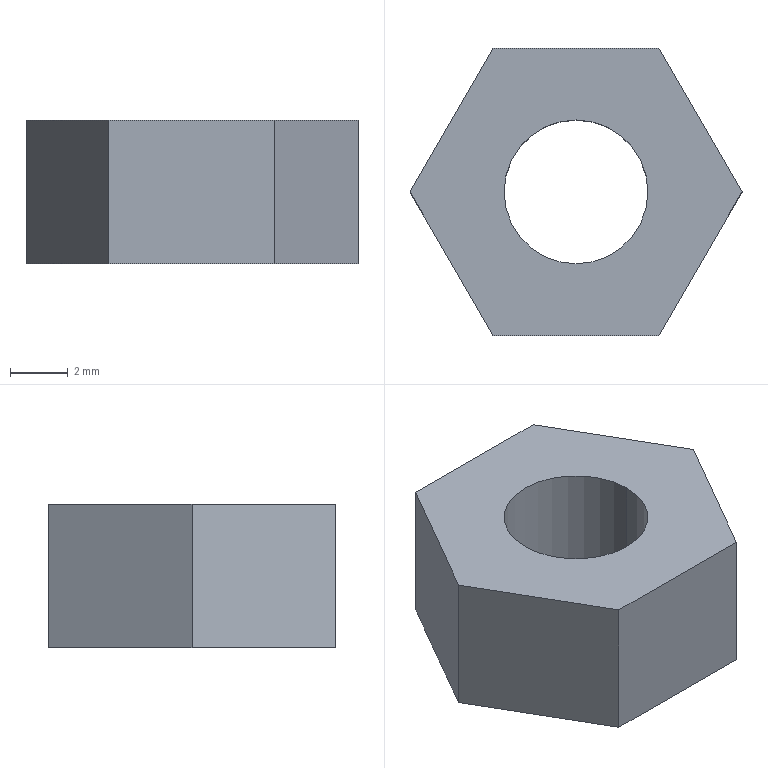Part | NX | 1 solid | 10 faces | box 11.547 x 10 x 5 mm | volume 334.838 mm3 | plane 8 | cylinder 2 | commonest cylinder face diameters 5 x2
STEP:
#1=CARTESIAN_POINT('',(2.887,5.,0.));
#2=VERTEX_POINT('',#1);
#3=CARTESIAN_POINT('',(5.774,0.,0.));
#4=VERTEX_POINT('',#3);
#5=CARTESIAN_POINT('',(2.887,5.,0.));
#6=DIRECTION('',(0.5,-0.866,0.));
#7=VECTOR('',#6,1000.);
#8=LINE('',#5,#7);
#9=EDGE_CURVE('',#2,#4,#8,.T.);
#10=ORIENTED_EDGE('',*,*,#9,.F.);
#11=CARTESIAN_POINT('',(-2.887,5.,0.));
#12=VERTEX_POINT('',#11);
#13=CARTESIAN_POINT('',(2.887,5.,0.));
#14=DIRECTION('',(-1.,0.,0.));
#15=VECTOR('',#14,1000.);
#16=LINE('',#13,#15);
#17=EDGE_CURVE('',#2,#12,#16,.T.);
#18=ORIENTED_EDGE('',*,*,#17,.T.);
#19=CARTESIAN_POINT('',(-5.774,0.,0.));
#20=VERTEX_POINT('',#19);
#21=CARTESIAN_POINT('',(-5.774,0.,0.));
#22=DIRECTION('',(0.5,0.866,0.));
#23=VECTOR('',#22,1000.);
#24=LINE('',#21,#23);
#25=EDGE_CURVE('',#20,#12,#24,.T.);
#26=ORIENTED_EDGE('',*,*,#25,.F.);
#27=CARTESIAN_POINT('',(-2.887,-5.,0.));
#28=VERTEX_POINT('',#27);
#29=CARTESIAN_POINT('',(-2.887,-5.,0.));
#30=DIRECTION('',(-0.5,0.866,0.));
#31=VECTOR('',#30,1000.);
#32=LINE('',#29,#31);
#33=EDGE_CURVE('',#28,#20,#32,.T.);
#34=ORIENTED_EDGE('',*,*,#33,.F.);
#35=CARTESIAN_POINT('',(2.887,-5.,0.));
#36=VERTEX_POINT('',#35);
#37=CARTESIAN_POINT('',(-2.887,-5.,0.));
#38=DIRECTION('',(1.,0.,0.));
#39=VECTOR('',#38,1000.);
#40=LINE('',#37,#39);
#41=EDGE_CURVE('',#28,#36,#40,.T.);
#42=ORIENTED_EDGE('',*,*,#41,.T.);
#43=CARTESIAN_POINT('',(5.774,0.,0.));
#44=DIRECTION('',(-0.5,-0.866,0.));
#45=VECTOR('',#44,1000.);
#46=LINE('',#43,#45);
#47=EDGE_CURVE('',#4,#36,#46,.T.);
#48=ORIENTED_EDGE('',*,*,#47,.F.);
#49=EDGE_LOOP('',(#10,#18,#26,#34,#42,#48));
#50=FACE_BOUND('',#49,.T.);
#51=CARTESIAN_POINT('',(-2.5,0.,0.));
#52=VERTEX_POINT('',#51);
#53=CARTESIAN_POINT('',(2.5,0.,0.));
#54=VERTEX_POINT('',#53);
#55=CARTESIAN_POINT('',(0.,0.,0.));
#56=DIRECTION('',(0.,0.,1.));
#57=DIRECTION('',(-1.,0.,0.));
#58=AXIS2_PLACEMENT_3D('',#55,#56,#57);
#59=CIRCLE('',#58,2.5);
#60=EDGE_CURVE('',#52,#54,#59,.T.);
#61=ORIENTED_EDGE('',*,*,#60,.F.);
#62=CARTESIAN_POINT('',(0.,0.,0.));
#63=DIRECTION('',(0.,0.,1.));
#64=DIRECTION('',(-1.,0.,0.));
#65=AXIS2_PLACEMENT_3D('',#62,#63,#64);
#66=CIRCLE('',#65,2.5);
#67=EDGE_CURVE('',#54,#52,#66,.T.);
#68=ORIENTED_EDGE('',*,*,#67,.F.);
#69=EDGE_LOOP('',(#61,#68));
#70=FACE_BOUND('',#69,.T.);
#71=CARTESIAN_POINT('',(0.,0.,0.));
#72=DIRECTION('',(0.,0.,-1.));
#73=DIRECTION('',(0.,-1.,0.));
#74=AXIS2_PLACEMENT_3D('',#71,#72,#73);
#75=PLANE('',#74);
#76=ADVANCED_FACE('',(#50,#70),#75,.F.);
#77=ORIENTED_EDGE('',*,*,#9,.T.);
#78=CARTESIAN_POINT('',(5.774,0.,-5.));
#79=VERTEX_POINT('',#78);
#80=CARTESIAN_POINT('',(5.774,0.,-5.));
#81=DIRECTION('',(0.,0.,1.));
#82=VECTOR('',#81,1000.);
#83=LINE('',#80,#82);
#84=EDGE_CURVE('',#79,#4,#83,.T.);
#85=ORIENTED_EDGE('',*,*,#84,.F.);
#86=CARTESIAN_POINT('',(2.887,5.,-5.));
#87=VERTEX_POINT('',#86);
#88=CARTESIAN_POINT('',(5.774,0.,-5.));
#89=DIRECTION('',(-0.5,0.866,0.));
#90=VECTOR('',#89,1000.);
#91=LINE('',#88,#90);
#92=EDGE_CURVE('',#79,#87,#91,.T.);
#93=ORIENTED_EDGE('',*,*,#92,.T.);
#94=CARTESIAN_POINT('',(2.887,5.,-5.));
#95=DIRECTION('',(0.,0.,1.));
#96=VECTOR('',#95,1000.);
#97=LINE('',#94,#96);
#98=EDGE_CURVE('',#87,#2,#97,.T.);
#99=ORIENTED_EDGE('',*,*,#98,.T.);
#100=EDGE_LOOP('',(#77,#85,#93,#99));
#101=FACE_BOUND('',#100,.T.);
#102=CARTESIAN_POINT('',(2.887,5.,0.));
#103=DIRECTION('',(0.866,0.5,0.));
#104=DIRECTION('',(0.,0.,-1.));
#105=AXIS2_PLACEMENT_3D('',#102,#103,#104);
#106=PLANE('',#105);
#107=ADVANCED_FACE('',(#101),#106,.T.);
#108=ORIENTED_EDGE('',*,*,#17,.F.);
#109=ORIENTED_EDGE('',*,*,#98,.F.);
#110=CARTESIAN_POINT('',(-2.887,5.,-5.));
#111=VERTEX_POINT('',#110);
#112=CARTESIAN_POINT('',(2.887,5.,-5.));
#113=DIRECTION('',(-1.,0.,0.));
#114=VECTOR('',#113,1000.);
#115=LINE('',#112,#114);
#116=EDGE_CURVE('',#87,#111,#115,.T.);
#117=ORIENTED_EDGE('',*,*,#116,.T.);
#118=CARTESIAN_POINT('',(-2.887,5.,-5.));
#119=DIRECTION('',(0.,0.,1.));
#120=VECTOR('',#119,1000.);
#121=LINE('',#118,#120);
#122=EDGE_CURVE('',#111,#12,#121,.T.);
#123=ORIENTED_EDGE('',*,*,#122,.T.);
#124=EDGE_LOOP('',(#108,#109,#117,#123));
#125=FACE_BOUND('',#124,.T.);
#126=CARTESIAN_POINT('',(-2.887,5.,0.));
#127=DIRECTION('',(0.,1.,0.));
#128=DIRECTION('',(1.,0.,0.));
#129=AXIS2_PLACEMENT_3D('',#126,#127,#128);
#130=PLANE('',#129);
#131=ADVANCED_FACE('',(#125),#130,.T.);
#132=ORIENTED_EDGE('',*,*,#25,.T.);
#133=ORIENTED_EDGE('',*,*,#122,.F.);
#134=CARTESIAN_POINT('',(-5.774,0.,-5.));
#135=VERTEX_POINT('',#134);
#136=CARTESIAN_POINT('',(-2.887,5.,-5.));
#137=DIRECTION('',(-0.5,-0.866,0.));
#138=VECTOR('',#137,1000.);
#139=LINE('',#136,#138);
#140=EDGE_CURVE('',#111,#135,#139,.T.);
#141=ORIENTED_EDGE('',*,*,#140,.T.);
#142=CARTESIAN_POINT('',(-5.774,0.,-5.));
#143=DIRECTION('',(0.,0.,1.));
#144=VECTOR('',#143,1000.);
#145=LINE('',#142,#144);
#146=EDGE_CURVE('',#135,#20,#145,.T.);
#147=ORIENTED_EDGE('',*,*,#146,.T.);
#148=EDGE_LOOP('',(#132,#133,#141,#147));
#149=FACE_BOUND('',#148,.T.);
#150=CARTESIAN_POINT('',(-5.774,0.,0.));
#151=DIRECTION('',(-0.866,0.5,0.));
#152=DIRECTION('',(0.,0.,1.));
#153=AXIS2_PLACEMENT_3D('',#150,#151,#152);
#154=PLANE('',#153);
#155=ADVANCED_FACE('',(#149),#154,.T.);
#156=ORIENTED_EDGE('',*,*,#33,.T.);
#157=ORIENTED_EDGE('',*,*,#146,.F.);
#158=CARTESIAN_POINT('',(-2.887,-5.,-5.));
#159=VERTEX_POINT('',#158);
#160=CARTESIAN_POINT('',(-5.774,0.,-5.));
#161=DIRECTION('',(0.5,-0.866,0.));
#162=VECTOR('',#161,1000.);
#163=LINE('',#160,#162);
#164=EDGE_CURVE('',#135,#159,#163,.T.);
#165=ORIENTED_EDGE('',*,*,#164,.T.);
#166=CARTESIAN_POINT('',(-2.887,-5.,-5.));
#167=DIRECTION('',(0.,0.,1.));
#168=VECTOR('',#167,1000.);
#169=LINE('',#166,#168);
#170=EDGE_CURVE('',#159,#28,#169,.T.);
#171=ORIENTED_EDGE('',*,*,#170,.T.);
#172=EDGE_LOOP('',(#156,#157,#165,#171));
#173=FACE_BOUND('',#172,.T.);
#174=CARTESIAN_POINT('',(-2.887,-5.,0.));
#175=DIRECTION('',(-0.866,-0.5,0.));
#176=DIRECTION('',(-0.5,0.866,0.));
#177=AXIS2_PLACEMENT_3D('',#174,#175,#176);
#178=PLANE('',#177);
#179=ADVANCED_FACE('',(#173),#178,.T.);
#180=ORIENTED_EDGE('',*,*,#41,.F.);
#181=ORIENTED_EDGE('',*,*,#170,.F.);
#182=CARTESIAN_POINT('',(2.887,-5.,-5.));
#183=VERTEX_POINT('',#182);
#184=CARTESIAN_POINT('',(-2.887,-5.,-5.));
#185=DIRECTION('',(1.,0.,0.));
#186=VECTOR('',#185,1000.);
#187=LINE('',#184,#186);
#188=EDGE_CURVE('',#159,#183,#187,.T.);
#189=ORIENTED_EDGE('',*,*,#188,.T.);
#190=CARTESIAN_POINT('',(2.887,-5.,-5.));
#191=DIRECTION('',(0.,0.,1.));
#192=VECTOR('',#191,1000.);
#193=LINE('',#190,#192);
#194=EDGE_CURVE('',#183,#36,#193,.T.);
#195=ORIENTED_EDGE('',*,*,#194,.T.);
#196=EDGE_LOOP('',(#180,#181,#189,#195));
#197=FACE_BOUND('',#196,.T.);
#198=CARTESIAN_POINT('',(2.887,-5.,0.));
#199=DIRECTION('',(0.,-1.,0.));
#200=DIRECTION('',(0.,0.,-1.));
#201=AXIS2_PLACEMENT_3D('',#198,#199,#200);
#202=PLANE('',#201);
#203=ADVANCED_FACE('',(#197),#202,.T.);
#204=ORIENTED_EDGE('',*,*,#47,.T.);
#205=ORIENTED_EDGE('',*,*,#194,.F.);
#206=CARTESIAN_POINT('',(2.887,-5.,-5.));
#207=DIRECTION('',(0.5,0.866,0.));
#208=VECTOR('',#207,1000.);
#209=LINE('',#206,#208);
#210=EDGE_CURVE('',#183,#79,#209,.T.);
#211=ORIENTED_EDGE('',*,*,#210,.T.);
#212=ORIENTED_EDGE('',*,*,#84,.T.);
#213=EDGE_LOOP('',(#204,#205,#211,#212));
#214=FACE_BOUND('',#213,.T.);
#215=CARTESIAN_POINT('',(5.774,0.,0.));
#216=DIRECTION('',(0.866,-0.5,0.));
#217=DIRECTION('',(0.,0.,-1.));
#218=AXIS2_PLACEMENT_3D('',#215,#216,#217);
#219=PLANE('',#218);
#220=ADVANCED_FACE('',(#214),#219,.T.);
#221=ORIENTED_EDGE('',*,*,#92,.F.);
#222=ORIENTED_EDGE('',*,*,#210,.F.);
#223=ORIENTED_EDGE('',*,*,#188,.F.);
#224=ORIENTED_EDGE('',*,*,#164,.F.);
#225=ORIENTED_EDGE('',*,*,#140,.F.);
#226=ORIENTED_EDGE('',*,*,#116,.F.);
#227=EDGE_LOOP('',(#221,#222,#223,#224,#225,#226));
#228=FACE_BOUND('',#227,.T.);
#229=CARTESIAN_POINT('',(2.5,0.,-5.));
#230=VERTEX_POINT('',#229);
#231=CARTESIAN_POINT('',(-2.5,0.,-5.));
#232=VERTEX_POINT('',#231);
#233=CARTESIAN_POINT('',(0.,0.,-5.));
#234=DIRECTION('',(0.,0.,-1.));
#235=DIRECTION('',(1.,0.,0.));
#236=AXIS2_PLACEMENT_3D('',#233,#234,#235);
#237=CIRCLE('',#236,2.5);
#238=EDGE_CURVE('',#230,#232,#237,.T.);
#239=ORIENTED_EDGE('',*,*,#238,.F.);
#240=CARTESIAN_POINT('',(0.,0.,-5.));
#241=DIRECTION('',(0.,0.,-1.));
#242=DIRECTION('',(1.,0.,0.));
#243=AXIS2_PLACEMENT_3D('',#240,#241,#242);
#244=CIRCLE('',#243,2.5);
#245=EDGE_CURVE('',#232,#230,#244,.T.);
#246=ORIENTED_EDGE('',*,*,#245,.F.);
#247=EDGE_LOOP('',(#239,#246));
#248=FACE_BOUND('',#247,.T.);
#249=CARTESIAN_POINT('',(0.,0.,-5.));
#250=DIRECTION('',(0.,0.,-1.));
#251=DIRECTION('',(0.,-1.,0.));
#252=AXIS2_PLACEMENT_3D('',#249,#250,#251);
#253=PLANE('',#252);
#254=ADVANCED_FACE('',(#228,#248),#253,.T.);
#255=ORIENTED_EDGE('',*,*,#60,.T.);
#256=CARTESIAN_POINT('',(2.5,0.,-5.));
#257=DIRECTION('',(0.,0.,1.));
#258=VECTOR('',#257,1000.);
#259=LINE('',#256,#258);
#260=EDGE_CURVE('',#230,#54,#259,.T.);
#261=ORIENTED_EDGE('',*,*,#260,.F.);
#262=ORIENTED_EDGE('',*,*,#238,.T.);
#263=CARTESIAN_POINT('',(-2.5,0.,-5.));
#264=DIRECTION('',(0.,0.,1.));
#265=VECTOR('',#264,1000.);
#266=LINE('',#263,#265);
#267=EDGE_CURVE('',#232,#52,#266,.T.);
#268=ORIENTED_EDGE('',*,*,#267,.T.);
#269=EDGE_LOOP('',(#255,#261,#262,#268));
#270=FACE_BOUND('',#269,.T.);
#271=CARTESIAN_POINT('',(0.,0.,-5.));
#272=DIRECTION('',(0.,0.,1.));
#273=DIRECTION('',(1.,0.,0.));
#274=AXIS2_PLACEMENT_3D('',#271,#272,#273);
#275=CYLINDRICAL_SURFACE('',#274,2.5);
#276=ADVANCED_FACE('',(#270),#275,.F.);
#277=ORIENTED_EDGE('',*,*,#260,.T.);
#278=ORIENTED_EDGE('',*,*,#67,.T.);
#279=ORIENTED_EDGE('',*,*,#267,.F.);
#280=ORIENTED_EDGE('',*,*,#245,.T.);
#281=EDGE_LOOP('',(#277,#278,#279,#280));
#282=FACE_BOUND('',#281,.T.);
#283=CARTESIAN_POINT('',(0.,0.,-5.));
#284=DIRECTION('',(0.,0.,1.));
#285=DIRECTION('',(1.,0.,0.));
#286=AXIS2_PLACEMENT_3D('',#283,#284,#285);
#287=CYLINDRICAL_SURFACE('',#286,2.5);
#288=ADVANCED_FACE('',(#282),#287,.F.);
#289=CLOSED_SHELL('',(#76,#107,#131,#155,#179,#203,#220,#254,#276,#288));
#290=MANIFOLD_SOLID_BREP('',#289);
#291=(LENGTH_UNIT()NAMED_UNIT(*)SI_UNIT(.MILLI.,.METRE.));
#292=UNCERTAINTY_MEASURE_WITH_UNIT(LENGTH_MEASURE(0.00001),#291,'','');
#293=(NAMED_UNIT(*)PLANE_ANGLE_UNIT()SI_UNIT($,.RADIAN.));
#294=(NAMED_UNIT(*)SI_UNIT($,.STERADIAN.)SOLID_ANGLE_UNIT());
#295=(GEOMETRIC_REPRESENTATION_CONTEXT(3)GLOBAL_UNCERTAINTY_ASSIGNED_CONTEXT((#292))GLOBAL_UNIT_ASSIGNED_CONTEXT((#291,#293,#294))REPRESENTATION_CONTEXT('',''));
#296=ADVANCED_BREP_SHAPE_REPRESENTATION('',(#290),#295);